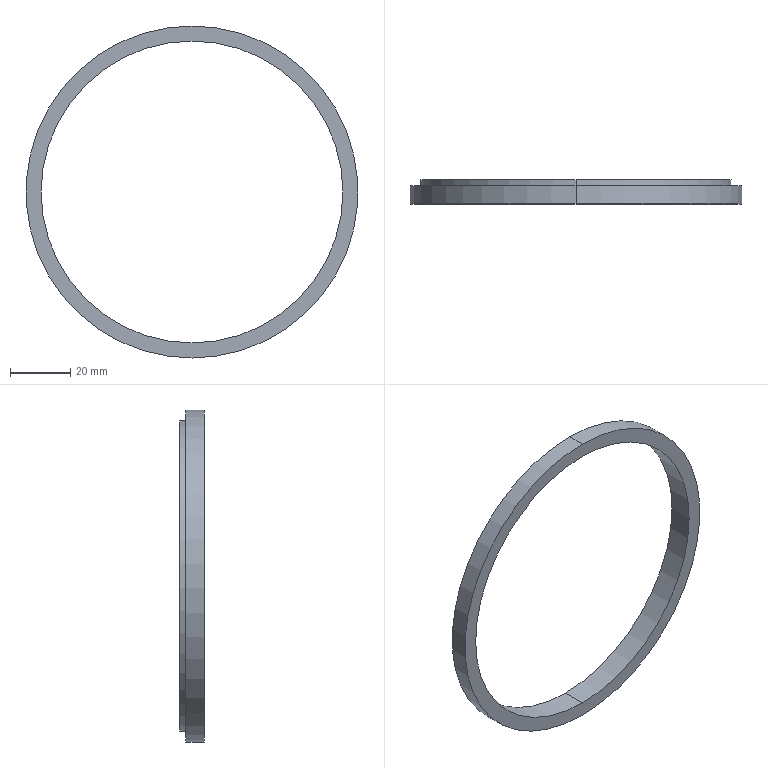Part | SolidWorks | features Extrusion 1, ICE 1 | 1 solid | 9 faces | box 110 x 8 x 110 mm | volume 10853 mm3 | cylinder 6 | plane 3 | commonest cylinder face diameters 100 x2 103 x2 110 x2
STEP:
#1=CARTESIAN_POINT('',(0.,8.,51.5));
#2=VERTEX_POINT('',#1);
#3=CARTESIAN_POINT('',(0.,8.,-51.5));
#4=VERTEX_POINT('',#3);
#5=CARTESIAN_POINT('',(0.,8.,0.));
#6=DIRECTION('',(0.,1.,0.));
#7=DIRECTION('',(0.,0.,1.));
#8=AXIS2_PLACEMENT_3D('',#5,#6,#7);
#9=CIRCLE('',#8,51.5);
#10=EDGE_CURVE('',#2,#4,#9,.T.);
#11=ORIENTED_EDGE('',*,*,#10,.F.);
#12=CARTESIAN_POINT('',(0.,6.,51.5));
#13=VERTEX_POINT('',#12);
#14=CARTESIAN_POINT('',(0.,8.,51.5));
#15=DIRECTION('',(0.,-1.,0.));
#16=VECTOR('',#15,1000.);
#17=LINE('',#14,#16);
#18=EDGE_CURVE('',#2,#13,#17,.T.);
#19=ORIENTED_EDGE('',*,*,#18,.T.);
#20=CARTESIAN_POINT('',(0.,6.,-51.5));
#21=VERTEX_POINT('',#20);
#22=CARTESIAN_POINT('',(0.,6.,0.));
#23=DIRECTION('',(0.,1.,0.));
#24=DIRECTION('',(0.,0.,1.));
#25=AXIS2_PLACEMENT_3D('',#22,#23,#24);
#26=CIRCLE('',#25,51.5);
#27=EDGE_CURVE('',#13,#21,#26,.T.);
#28=ORIENTED_EDGE('',*,*,#27,.T.);
#29=CARTESIAN_POINT('',(0.,8.,-51.5));
#30=DIRECTION('',(0.,-1.,0.));
#31=VECTOR('',#30,1000.);
#32=LINE('',#29,#31);
#33=EDGE_CURVE('',#4,#21,#32,.T.);
#34=ORIENTED_EDGE('',*,*,#33,.F.);
#35=EDGE_LOOP('',(#11,#19,#28,#34));
#36=FACE_OUTER_BOUND('',#35,.T.);
#37=CARTESIAN_POINT('',(0.,8.,0.));
#38=DIRECTION('',(0.,-1.,0.));
#39=DIRECTION('',(0.,0.,-1.));
#40=AXIS2_PLACEMENT_3D('',#37,#38,#39);
#41=CYLINDRICAL_SURFACE('',#40,51.5);
#42=ADVANCED_FACE('',(#36),#41,.T.);
#43=CARTESIAN_POINT('',(0.,8.,-50.));
#44=VERTEX_POINT('',#43);
#45=CARTESIAN_POINT('',(0.,8.,50.));
#46=VERTEX_POINT('',#45);
#47=CARTESIAN_POINT('',(0.,8.,0.));
#48=DIRECTION('',(0.,1.,0.));
#49=DIRECTION('',(0.,0.,1.));
#50=AXIS2_PLACEMENT_3D('',#47,#48,#49);
#51=CIRCLE('',#50,50.);
#52=EDGE_CURVE('',#44,#46,#51,.T.);
#53=ORIENTED_EDGE('',*,*,#52,.T.);
#54=CARTESIAN_POINT('',(0.,0.,50.));
#55=VERTEX_POINT('',#54);
#56=CARTESIAN_POINT('',(0.,6.,50.));
#57=DIRECTION('',(0.,-1.,0.));
#58=VECTOR('',#57,1000.);
#59=LINE('',#56,#58);
#60=EDGE_CURVE('',#46,#55,#59,.T.);
#61=ORIENTED_EDGE('',*,*,#60,.T.);
#62=CARTESIAN_POINT('',(0.,0.,-50.));
#63=VERTEX_POINT('',#62);
#64=CARTESIAN_POINT('',(0.,0.,0.));
#65=DIRECTION('',(0.,1.,0.));
#66=DIRECTION('',(0.,0.,1.));
#67=AXIS2_PLACEMENT_3D('',#64,#65,#66);
#68=CIRCLE('',#67,50.);
#69=EDGE_CURVE('',#63,#55,#68,.T.);
#70=ORIENTED_EDGE('',*,*,#69,.F.);
#71=CARTESIAN_POINT('',(0.,6.,-50.));
#72=DIRECTION('',(0.,-1.,0.));
#73=VECTOR('',#72,1000.);
#74=LINE('',#71,#73);
#75=EDGE_CURVE('',#44,#63,#74,.T.);
#76=ORIENTED_EDGE('',*,*,#75,.F.);
#77=EDGE_LOOP('',(#53,#61,#70,#76));
#78=FACE_OUTER_BOUND('',#77,.T.);
#79=CARTESIAN_POINT('',(0.,6.,0.));
#80=DIRECTION('',(0.,-1.,0.));
#81=DIRECTION('',(0.,0.,-1.));
#82=AXIS2_PLACEMENT_3D('',#79,#80,#81);
#83=CYLINDRICAL_SURFACE('',#82,50.);
#84=ADVANCED_FACE('',(#78),#83,.F.);
#85=CARTESIAN_POINT('',(0.,6.,55.));
#86=VERTEX_POINT('',#85);
#87=CARTESIAN_POINT('',(0.,6.,-55.));
#88=VERTEX_POINT('',#87);
#89=CARTESIAN_POINT('',(0.,6.,0.));
#90=DIRECTION('',(0.,1.,0.));
#91=DIRECTION('',(0.,0.,1.));
#92=AXIS2_PLACEMENT_3D('',#89,#90,#91);
#93=CIRCLE('',#92,55.);
#94=EDGE_CURVE('',#86,#88,#93,.T.);
#95=ORIENTED_EDGE('',*,*,#94,.F.);
#96=CARTESIAN_POINT('',(0.,0.,55.));
#97=VERTEX_POINT('',#96);
#98=CARTESIAN_POINT('',(0.,6.,55.));
#99=DIRECTION('',(0.,-1.,0.));
#100=VECTOR('',#99,1000.);
#101=LINE('',#98,#100);
#102=EDGE_CURVE('',#86,#97,#101,.T.);
#103=ORIENTED_EDGE('',*,*,#102,.T.);
#104=CARTESIAN_POINT('',(0.,0.,-55.));
#105=VERTEX_POINT('',#104);
#106=CARTESIAN_POINT('',(0.,0.,0.));
#107=DIRECTION('',(0.,1.,0.));
#108=DIRECTION('',(0.,0.,1.));
#109=AXIS2_PLACEMENT_3D('',#106,#107,#108);
#110=CIRCLE('',#109,55.);
#111=EDGE_CURVE('',#97,#105,#110,.T.);
#112=ORIENTED_EDGE('',*,*,#111,.T.);
#113=CARTESIAN_POINT('',(0.,6.,-55.));
#114=DIRECTION('',(0.,-1.,0.));
#115=VECTOR('',#114,1000.);
#116=LINE('',#113,#115);
#117=EDGE_CURVE('',#88,#105,#116,.T.);
#118=ORIENTED_EDGE('',*,*,#117,.F.);
#119=EDGE_LOOP('',(#95,#103,#112,#118));
#120=FACE_OUTER_BOUND('',#119,.T.);
#121=CARTESIAN_POINT('',(0.,6.,0.));
#122=DIRECTION('',(0.,-1.,0.));
#123=DIRECTION('',(0.,0.,-1.));
#124=AXIS2_PLACEMENT_3D('',#121,#122,#123);
#125=CYLINDRICAL_SURFACE('',#124,55.);
#126=ADVANCED_FACE('',(#120),#125,.T.);
#127=CARTESIAN_POINT('',(0.,6.,0.));
#128=DIRECTION('',(0.,1.,0.));
#129=DIRECTION('',(0.,0.,1.));
#130=AXIS2_PLACEMENT_3D('',#127,#128,#129);
#131=CIRCLE('',#130,55.);
#132=EDGE_CURVE('',#88,#86,#131,.T.);
#133=ORIENTED_EDGE('',*,*,#132,.T.);
#134=ORIENTED_EDGE('',*,*,#94,.T.);
#135=EDGE_LOOP('',(#133,#134));
#136=FACE_OUTER_BOUND('',#135,.T.);
#137=CARTESIAN_POINT('',(0.,6.,0.));
#138=DIRECTION('',(0.,1.,0.));
#139=DIRECTION('',(0.,0.,1.));
#140=AXIS2_PLACEMENT_3D('',#137,#138,#139);
#141=CIRCLE('',#140,51.5);
#142=EDGE_CURVE('',#21,#13,#141,.T.);
#143=ORIENTED_EDGE('',*,*,#142,.F.);
#144=ORIENTED_EDGE('',*,*,#27,.F.);
#145=EDGE_LOOP('',(#143,#144));
#146=FACE_BOUND('',#145,.T.);
#147=CARTESIAN_POINT('',(0.,6.,0.));
#148=DIRECTION('',(0.,1.,0.));
#149=DIRECTION('',(0.,0.,1.));
#150=AXIS2_PLACEMENT_3D('',#147,#148,#149);
#151=PLANE('',#150);
#152=ADVANCED_FACE('',(#136,#146),#151,.T.);
#153=CARTESIAN_POINT('',(0.,0.,0.));
#154=DIRECTION('',(0.,1.,0.));
#155=DIRECTION('',(0.,0.,1.));
#156=AXIS2_PLACEMENT_3D('',#153,#154,#155);
#157=CIRCLE('',#156,55.);
#158=EDGE_CURVE('',#105,#97,#157,.T.);
#159=ORIENTED_EDGE('',*,*,#158,.F.);
#160=ORIENTED_EDGE('',*,*,#111,.F.);
#161=EDGE_LOOP('',(#159,#160));
#162=FACE_OUTER_BOUND('',#161,.T.);
#163=ORIENTED_EDGE('',*,*,#69,.T.);
#164=CARTESIAN_POINT('',(0.,0.,0.));
#165=DIRECTION('',(0.,1.,0.));
#166=DIRECTION('',(0.,0.,1.));
#167=AXIS2_PLACEMENT_3D('',#164,#165,#166);
#168=CIRCLE('',#167,50.);
#169=EDGE_CURVE('',#55,#63,#168,.T.);
#170=ORIENTED_EDGE('',*,*,#169,.T.);
#171=EDGE_LOOP('',(#163,#170));
#172=FACE_BOUND('',#171,.T.);
#173=CARTESIAN_POINT('',(0.,0.,0.));
#174=DIRECTION('',(0.,1.,0.));
#175=DIRECTION('',(0.,0.,1.));
#176=AXIS2_PLACEMENT_3D('',#173,#174,#175);
#177=PLANE('',#176);
#178=ADVANCED_FACE('',(#162,#172),#177,.F.);
#179=ORIENTED_EDGE('',*,*,#102,.F.);
#180=ORIENTED_EDGE('',*,*,#132,.F.);
#181=ORIENTED_EDGE('',*,*,#117,.T.);
#182=ORIENTED_EDGE('',*,*,#158,.T.);
#183=EDGE_LOOP('',(#179,#180,#181,#182));
#184=FACE_OUTER_BOUND('',#183,.T.);
#185=CARTESIAN_POINT('',(0.,6.,0.));
#186=DIRECTION('',(0.,-1.,0.));
#187=DIRECTION('',(0.,0.,-1.));
#188=AXIS2_PLACEMENT_3D('',#185,#186,#187);
#189=CYLINDRICAL_SURFACE('',#188,55.);
#190=ADVANCED_FACE('',(#184),#189,.T.);
#191=ORIENTED_EDGE('',*,*,#60,.F.);
#192=CARTESIAN_POINT('',(0.,8.,0.));
#193=DIRECTION('',(0.,1.,0.));
#194=DIRECTION('',(0.,0.,1.));
#195=AXIS2_PLACEMENT_3D('',#192,#193,#194);
#196=CIRCLE('',#195,50.);
#197=EDGE_CURVE('',#46,#44,#196,.T.);
#198=ORIENTED_EDGE('',*,*,#197,.T.);
#199=ORIENTED_EDGE('',*,*,#75,.T.);
#200=ORIENTED_EDGE('',*,*,#169,.F.);
#201=EDGE_LOOP('',(#191,#198,#199,#200));
#202=FACE_OUTER_BOUND('',#201,.T.);
#203=CARTESIAN_POINT('',(0.,6.,0.));
#204=DIRECTION('',(0.,-1.,0.));
#205=DIRECTION('',(0.,0.,-1.));
#206=AXIS2_PLACEMENT_3D('',#203,#204,#205);
#207=CYLINDRICAL_SURFACE('',#206,50.);
#208=ADVANCED_FACE('',(#202),#207,.F.);
#209=CARTESIAN_POINT('',(0.,8.,0.));
#210=DIRECTION('',(0.,1.,0.));
#211=DIRECTION('',(0.,0.,1.));
#212=AXIS2_PLACEMENT_3D('',#209,#210,#211);
#213=CIRCLE('',#212,51.5);
#214=EDGE_CURVE('',#4,#2,#213,.T.);
#215=ORIENTED_EDGE('',*,*,#214,.T.);
#216=ORIENTED_EDGE('',*,*,#10,.T.);
#217=EDGE_LOOP('',(#215,#216));
#218=FACE_OUTER_BOUND('',#217,.T.);
#219=ORIENTED_EDGE('',*,*,#52,.F.);
#220=ORIENTED_EDGE('',*,*,#197,.F.);
#221=EDGE_LOOP('',(#219,#220));
#222=FACE_BOUND('',#221,.T.);
#223=CARTESIAN_POINT('',(0.,8.,0.));
#224=DIRECTION('',(0.,1.,0.));
#225=DIRECTION('',(0.,0.,1.));
#226=AXIS2_PLACEMENT_3D('',#223,#224,#225);
#227=PLANE('',#226);
#228=ADVANCED_FACE('',(#218,#222),#227,.T.);
#229=ORIENTED_EDGE('',*,*,#18,.F.);
#230=ORIENTED_EDGE('',*,*,#214,.F.);
#231=ORIENTED_EDGE('',*,*,#33,.T.);
#232=ORIENTED_EDGE('',*,*,#142,.T.);
#233=EDGE_LOOP('',(#229,#230,#231,#232));
#234=FACE_OUTER_BOUND('',#233,.T.);
#235=CARTESIAN_POINT('',(0.,8.,0.));
#236=DIRECTION('',(0.,-1.,0.));
#237=DIRECTION('',(0.,0.,-1.));
#238=AXIS2_PLACEMENT_3D('',#235,#236,#237);
#239=CYLINDRICAL_SURFACE('',#238,51.5);
#240=ADVANCED_FACE('',(#234),#239,.T.);
#241=CLOSED_SHELL('',(#42,#84,#126,#152,#178,#190,#208,#228,#240));
#242=MANIFOLD_SOLID_BREP('',#241);
#243=CARTESIAN_POINT('',(0.,0.,0.));
#244=DIRECTION('',(0.,0.,1.));
#245=DIRECTION('',(1.,0.,0.));
#246=AXIS2_PLACEMENT_3D('',#243,#244,#245);
#247=(LENGTH_UNIT()NAMED_UNIT(*)SI_UNIT(.MILLI.,.METRE.));
#248=UNCERTAINTY_MEASURE_WITH_UNIT(LENGTH_MEASURE(0.00001),#247,'','');
#249=(NAMED_UNIT(*)PLANE_ANGLE_UNIT()SI_UNIT($,.RADIAN.));
#250=(NAMED_UNIT(*)SI_UNIT($,.STERADIAN.)SOLID_ANGLE_UNIT());
#251=(GEOMETRIC_REPRESENTATION_CONTEXT(3)GLOBAL_UNCERTAINTY_ASSIGNED_CONTEXT((#248))GLOBAL_UNIT_ASSIGNED_CONTEXT((#247,#249,#250))REPRESENTATION_CONTEXT('',''));
#252=ADVANCED_BREP_SHAPE_REPRESENTATION('',(#242,#246),#251);